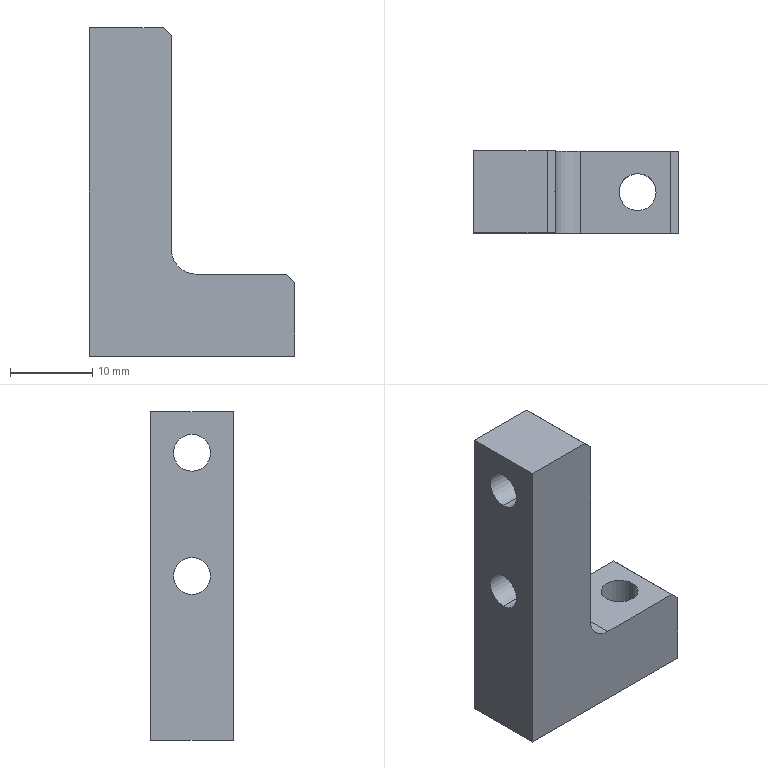Part | SolidWorks | features HoleWzd 2, Chamfer 1, Extrusion 1, ICE 1 | 1 solid | 23 faces | box 25 x 10 x 40 mm | volume 4716 mm3 | plane 12 | cylinder 11 | commonest cylinder face diameters 4.5 x6 8 x4 6 x1
STEP:
#1=CARTESIAN_POINT('',(5.25,0.,-20.));
#2=VERTEX_POINT('',#1);
#3=CARTESIAN_POINT('',(9.75,0.,-20.));
#4=VERTEX_POINT('',#3);
#5=CARTESIAN_POINT('',(7.5,0.,-20.));
#6=DIRECTION('',(0.,0.,1.));
#7=DIRECTION('',(1.,0.,0.));
#8=AXIS2_PLACEMENT_3D('',#5,#6,#7);
#9=CIRCLE('',#8,2.25);
#10=EDGE_CURVE('',#2,#4,#9,.T.);
#11=ORIENTED_EDGE('',*,*,#10,.F.);
#12=CARTESIAN_POINT('',(5.25,0.,-10.));
#13=VERTEX_POINT('',#12);
#14=CARTESIAN_POINT('',(5.25,0.,-10.));
#15=DIRECTION('',(0.,0.,1.));
#16=VECTOR('',#15,1000.);
#17=LINE('',#14,#16);
#18=EDGE_CURVE('',#2,#13,#17,.T.);
#19=ORIENTED_EDGE('',*,*,#18,.T.);
#20=CARTESIAN_POINT('',(9.75,0.,-10.));
#21=VERTEX_POINT('',#20);
#22=CARTESIAN_POINT('',(7.5,0.,-10.));
#23=DIRECTION('',(0.,0.,1.));
#24=DIRECTION('',(1.,0.,0.));
#25=AXIS2_PLACEMENT_3D('',#22,#23,#24);
#26=CIRCLE('',#25,2.25);
#27=EDGE_CURVE('',#13,#21,#26,.T.);
#28=ORIENTED_EDGE('',*,*,#27,.T.);
#29=CARTESIAN_POINT('',(9.75,0.,-10.));
#30=DIRECTION('',(0.,0.,1.));
#31=VECTOR('',#30,1000.);
#32=LINE('',#29,#31);
#33=EDGE_CURVE('',#4,#21,#32,.T.);
#34=ORIENTED_EDGE('',*,*,#33,.F.);
#35=EDGE_LOOP('',(#11,#19,#28,#34));
#36=FACE_OUTER_BOUND('',#35,.T.);
#37=CARTESIAN_POINT('',(7.5,0.,-10.));
#38=DIRECTION('',(0.,0.,1.));
#39=DIRECTION('',(1.,0.,0.));
#40=AXIS2_PLACEMENT_3D('',#37,#38,#39);
#41=CYLINDRICAL_SURFACE('',#40,2.25);
#42=ADVANCED_FACE('',(#36),#41,.F.);
#43=CARTESIAN_POINT('',(-7.1,0.,19.));
#44=VERTEX_POINT('',#43);
#45=CARTESIAN_POINT('',(-7.1,0.,11.));
#46=VERTEX_POINT('',#45);
#47=CARTESIAN_POINT('',(-7.1,0.,15.));
#48=DIRECTION('',(1.,0.,0.));
#49=DIRECTION('',(0.,0.,-1.));
#50=AXIS2_PLACEMENT_3D('',#47,#48,#49);
#51=CIRCLE('',#50,4.);
#52=EDGE_CURVE('',#44,#46,#51,.T.);
#53=ORIENTED_EDGE('',*,*,#52,.F.);
#54=CARTESIAN_POINT('',(-2.5,0.,19.));
#55=VERTEX_POINT('',#54);
#56=CARTESIAN_POINT('',(-2.5,0.,19.));
#57=DIRECTION('',(1.,0.,0.));
#58=VECTOR('',#57,1000.);
#59=LINE('',#56,#58);
#60=EDGE_CURVE('',#44,#55,#59,.T.);
#61=ORIENTED_EDGE('',*,*,#60,.T.);
#62=CARTESIAN_POINT('',(-2.5,0.,11.));
#63=VERTEX_POINT('',#62);
#64=CARTESIAN_POINT('',(-2.5,0.,15.));
#65=DIRECTION('',(1.,0.,0.));
#66=DIRECTION('',(0.,0.,-1.));
#67=AXIS2_PLACEMENT_3D('',#64,#65,#66);
#68=CIRCLE('',#67,4.);
#69=EDGE_CURVE('',#55,#63,#68,.T.);
#70=ORIENTED_EDGE('',*,*,#69,.T.);
#71=CARTESIAN_POINT('',(-2.5,0.,11.));
#72=DIRECTION('',(1.,0.,0.));
#73=VECTOR('',#72,1000.);
#74=LINE('',#71,#73);
#75=EDGE_CURVE('',#46,#63,#74,.T.);
#76=ORIENTED_EDGE('',*,*,#75,.F.);
#77=EDGE_LOOP('',(#53,#61,#70,#76));
#78=FACE_OUTER_BOUND('',#77,.T.);
#79=CARTESIAN_POINT('',(-2.5,0.,15.));
#80=DIRECTION('',(1.,0.,0.));
#81=DIRECTION('',(0.,0.,-1.));
#82=AXIS2_PLACEMENT_3D('',#79,#80,#81);
#83=CYLINDRICAL_SURFACE('',#82,4.);
#84=ADVANCED_FACE('',(#78),#83,.F.);
#85=CARTESIAN_POINT('',(-12.5,0.,17.25));
#86=VERTEX_POINT('',#85);
#87=CARTESIAN_POINT('',(-12.5,0.,12.75));
#88=VERTEX_POINT('',#87);
#89=CARTESIAN_POINT('',(-12.5,0.,15.));
#90=DIRECTION('',(1.,0.,0.));
#91=DIRECTION('',(0.,0.,-1.));
#92=AXIS2_PLACEMENT_3D('',#89,#90,#91);
#93=CIRCLE('',#92,2.25);
#94=EDGE_CURVE('',#86,#88,#93,.T.);
#95=ORIENTED_EDGE('',*,*,#94,.F.);
#96=CARTESIAN_POINT('',(-7.1,0.,17.25));
#97=VERTEX_POINT('',#96);
#98=CARTESIAN_POINT('',(-2.5,0.,17.25));
#99=DIRECTION('',(1.,0.,0.));
#100=VECTOR('',#99,1000.);
#101=LINE('',#98,#100);
#102=EDGE_CURVE('',#86,#97,#101,.T.);
#103=ORIENTED_EDGE('',*,*,#102,.T.);
#104=CARTESIAN_POINT('',(-7.1,0.,12.75));
#105=VERTEX_POINT('',#104);
#106=CARTESIAN_POINT('',(-7.1,0.,15.));
#107=DIRECTION('',(1.,0.,0.));
#108=DIRECTION('',(0.,0.,-1.));
#109=AXIS2_PLACEMENT_3D('',#106,#107,#108);
#110=CIRCLE('',#109,2.25);
#111=EDGE_CURVE('',#97,#105,#110,.T.);
#112=ORIENTED_EDGE('',*,*,#111,.T.);
#113=CARTESIAN_POINT('',(-2.5,0.,12.75));
#114=DIRECTION('',(1.,0.,0.));
#115=VECTOR('',#114,1000.);
#116=LINE('',#113,#115);
#117=EDGE_CURVE('',#88,#105,#116,.T.);
#118=ORIENTED_EDGE('',*,*,#117,.F.);
#119=EDGE_LOOP('',(#95,#103,#112,#118));
#120=FACE_OUTER_BOUND('',#119,.T.);
#121=CARTESIAN_POINT('',(-2.5,0.,15.));
#122=DIRECTION('',(1.,0.,0.));
#123=DIRECTION('',(0.,0.,-1.));
#124=AXIS2_PLACEMENT_3D('',#121,#122,#123);
#125=CYLINDRICAL_SURFACE('',#124,2.25);
#126=ADVANCED_FACE('',(#120),#125,.F.);
#127=CARTESIAN_POINT('',(-7.1,0.,4.));
#128=VERTEX_POINT('',#127);
#129=CARTESIAN_POINT('',(-7.1,0.,-4.));
#130=VERTEX_POINT('',#129);
#131=CARTESIAN_POINT('',(-7.1,0.,0.));
#132=DIRECTION('',(1.,0.,0.));
#133=DIRECTION('',(0.,0.,-1.));
#134=AXIS2_PLACEMENT_3D('',#131,#132,#133);
#135=CIRCLE('',#134,4.);
#136=EDGE_CURVE('',#128,#130,#135,.T.);
#137=ORIENTED_EDGE('',*,*,#136,.F.);
#138=CARTESIAN_POINT('',(-2.5,0.,4.));
#139=VERTEX_POINT('',#138);
#140=CARTESIAN_POINT('',(-2.5,0.,4.));
#141=DIRECTION('',(1.,0.,0.));
#142=VECTOR('',#141,1000.);
#143=LINE('',#140,#142);
#144=EDGE_CURVE('',#128,#139,#143,.T.);
#145=ORIENTED_EDGE('',*,*,#144,.T.);
#146=CARTESIAN_POINT('',(-2.5,0.,-4.));
#147=VERTEX_POINT('',#146);
#148=CARTESIAN_POINT('',(-2.5,0.,0.));
#149=DIRECTION('',(1.,0.,0.));
#150=DIRECTION('',(0.,0.,-1.));
#151=AXIS2_PLACEMENT_3D('',#148,#149,#150);
#152=CIRCLE('',#151,4.);
#153=EDGE_CURVE('',#139,#147,#152,.T.);
#154=ORIENTED_EDGE('',*,*,#153,.T.);
#155=CARTESIAN_POINT('',(-2.5,0.,-4.));
#156=DIRECTION('',(1.,0.,0.));
#157=VECTOR('',#156,1000.);
#158=LINE('',#155,#157);
#159=EDGE_CURVE('',#130,#147,#158,.T.);
#160=ORIENTED_EDGE('',*,*,#159,.F.);
#161=EDGE_LOOP('',(#137,#145,#154,#160));
#162=FACE_OUTER_BOUND('',#161,.T.);
#163=CARTESIAN_POINT('',(-2.5,0.,0.));
#164=DIRECTION('',(1.,0.,0.));
#165=DIRECTION('',(0.,0.,-1.));
#166=AXIS2_PLACEMENT_3D('',#163,#164,#165);
#167=CYLINDRICAL_SURFACE('',#166,4.);
#168=ADVANCED_FACE('',(#162),#167,.F.);
#169=CARTESIAN_POINT('',(-12.5,0.,2.25));
#170=VERTEX_POINT('',#169);
#171=CARTESIAN_POINT('',(-12.5,0.,-2.25));
#172=VERTEX_POINT('',#171);
#173=CARTESIAN_POINT('',(-12.5,0.,0.));
#174=DIRECTION('',(1.,0.,0.));
#175=DIRECTION('',(0.,0.,-1.));
#176=AXIS2_PLACEMENT_3D('',#173,#174,#175);
#177=CIRCLE('',#176,2.25);
#178=EDGE_CURVE('',#170,#172,#177,.T.);
#179=ORIENTED_EDGE('',*,*,#178,.F.);
#180=CARTESIAN_POINT('',(-7.1,0.,2.25));
#181=VERTEX_POINT('',#180);
#182=CARTESIAN_POINT('',(-2.5,0.,2.25));
#183=DIRECTION('',(1.,0.,0.));
#184=VECTOR('',#183,1000.);
#185=LINE('',#182,#184);
#186=EDGE_CURVE('',#170,#181,#185,.T.);
#187=ORIENTED_EDGE('',*,*,#186,.T.);
#188=CARTESIAN_POINT('',(-7.1,0.,-2.25));
#189=VERTEX_POINT('',#188);
#190=CARTESIAN_POINT('',(-7.1,0.,0.));
#191=DIRECTION('',(1.,0.,0.));
#192=DIRECTION('',(0.,0.,-1.));
#193=AXIS2_PLACEMENT_3D('',#190,#191,#192);
#194=CIRCLE('',#193,2.25);
#195=EDGE_CURVE('',#181,#189,#194,.T.);
#196=ORIENTED_EDGE('',*,*,#195,.T.);
#197=CARTESIAN_POINT('',(-2.5,0.,-2.25));
#198=DIRECTION('',(1.,0.,0.));
#199=VECTOR('',#198,1000.);
#200=LINE('',#197,#199);
#201=EDGE_CURVE('',#172,#189,#200,.T.);
#202=ORIENTED_EDGE('',*,*,#201,.F.);
#203=EDGE_LOOP('',(#179,#187,#196,#202));
#204=FACE_OUTER_BOUND('',#203,.T.);
#205=CARTESIAN_POINT('',(-2.5,0.,0.));
#206=DIRECTION('',(1.,0.,0.));
#207=DIRECTION('',(0.,0.,-1.));
#208=AXIS2_PLACEMENT_3D('',#205,#206,#207);
#209=CYLINDRICAL_SURFACE('',#208,2.25);
#210=ADVANCED_FACE('',(#204),#209,.F.);
#211=CARTESIAN_POINT('',(12.5,5.,-11.));
#212=VERTEX_POINT('',#211);
#213=CARTESIAN_POINT('',(12.5,5.,-20.));
#214=VERTEX_POINT('',#213);
#215=CARTESIAN_POINT('',(12.5,5.,20.));
#216=DIRECTION('',(0.,0.,-1.));
#217=VECTOR('',#216,1000.);
#218=LINE('',#215,#217);
#219=EDGE_CURVE('',#212,#214,#218,.T.);
#220=ORIENTED_EDGE('',*,*,#219,.F.);
#221=CARTESIAN_POINT('',(12.5,-5.,-11.));
#222=VERTEX_POINT('',#221);
#223=CARTESIAN_POINT('',(12.5,5.,-11.));
#224=DIRECTION('',(0.,-1.,0.));
#225=VECTOR('',#224,1000.);
#226=LINE('',#223,#225);
#227=EDGE_CURVE('',#212,#222,#226,.T.);
#228=ORIENTED_EDGE('',*,*,#227,.T.);
#229=CARTESIAN_POINT('',(12.5,-5.,-20.));
#230=VERTEX_POINT('',#229);
#231=CARTESIAN_POINT('',(12.5,-5.,20.));
#232=DIRECTION('',(0.,0.,-1.));
#233=VECTOR('',#232,1000.);
#234=LINE('',#231,#233);
#235=EDGE_CURVE('',#222,#230,#234,.T.);
#236=ORIENTED_EDGE('',*,*,#235,.T.);
#237=CARTESIAN_POINT('',(12.5,5.,-20.));
#238=DIRECTION('',(0.,-1.,0.));
#239=VECTOR('',#238,1000.);
#240=LINE('',#237,#239);
#241=EDGE_CURVE('',#214,#230,#240,.T.);
#242=ORIENTED_EDGE('',*,*,#241,.F.);
#243=EDGE_LOOP('',(#220,#228,#236,#242));
#244=FACE_OUTER_BOUND('',#243,.T.);
#245=CARTESIAN_POINT('',(12.5,5.,20.));
#246=DIRECTION('',(-1.,0.,0.));
#247=DIRECTION('',(0.,0.,1.));
#248=AXIS2_PLACEMENT_3D('',#245,#246,#247);
#249=PLANE('',#248);
#250=ADVANCED_FACE('',(#244),#249,.F.);
#251=CARTESIAN_POINT('',(7.5,0.,-20.));
#252=DIRECTION('',(0.,0.,1.));
#253=DIRECTION('',(1.,0.,0.));
#254=AXIS2_PLACEMENT_3D('',#251,#252,#253);
#255=CIRCLE('',#254,2.25);
#256=EDGE_CURVE('',#4,#2,#255,.T.);
#257=ORIENTED_EDGE('',*,*,#256,.T.);
#258=ORIENTED_EDGE('',*,*,#10,.T.);
#259=EDGE_LOOP('',(#257,#258));
#260=FACE_BOUND('',#259,.T.);
#261=CARTESIAN_POINT('',(-12.5,-5.,-20.));
#262=VERTEX_POINT('',#261);
#263=CARTESIAN_POINT('',(-12.5,-5.,-20.));
#264=DIRECTION('',(-1.,0.,0.));
#265=VECTOR('',#264,1000.);
#266=LINE('',#263,#265);
#267=EDGE_CURVE('',#230,#262,#266,.T.);
#268=ORIENTED_EDGE('',*,*,#267,.T.);
#269=CARTESIAN_POINT('',(-12.5,5.,-20.));
#270=VERTEX_POINT('',#269);
#271=CARTESIAN_POINT('',(-12.5,5.,-20.));
#272=DIRECTION('',(0.,-1.,0.));
#273=VECTOR('',#272,1000.);
#274=LINE('',#271,#273);
#275=EDGE_CURVE('',#270,#262,#274,.T.);
#276=ORIENTED_EDGE('',*,*,#275,.F.);
#277=CARTESIAN_POINT('',(-12.5,5.,-20.));
#278=DIRECTION('',(-1.,0.,0.));
#279=VECTOR('',#278,1000.);
#280=LINE('',#277,#279);
#281=EDGE_CURVE('',#214,#270,#280,.T.);
#282=ORIENTED_EDGE('',*,*,#281,.F.);
#283=ORIENTED_EDGE('',*,*,#241,.T.);
#284=EDGE_LOOP('',(#268,#276,#282,#283));
#285=FACE_OUTER_BOUND('',#284,.T.);
#286=CARTESIAN_POINT('',(-12.5,5.,-20.));
#287=DIRECTION('',(0.,0.,1.));
#288=DIRECTION('',(1.,0.,0.));
#289=AXIS2_PLACEMENT_3D('',#286,#287,#288);
#290=PLANE('',#289);
#291=ADVANCED_FACE('',(#260,#285),#290,.F.);
#292=CARTESIAN_POINT('',(-12.5,0.,15.));
#293=DIRECTION('',(1.,0.,0.));
#294=DIRECTION('',(0.,0.,-1.));
#295=AXIS2_PLACEMENT_3D('',#292,#293,#294);
#296=CIRCLE('',#295,2.25);
#297=EDGE_CURVE('',#88,#86,#296,.T.);
#298=ORIENTED_EDGE('',*,*,#297,.T.);
#299=ORIENTED_EDGE('',*,*,#94,.T.);
#300=EDGE_LOOP('',(#298,#299));
#301=FACE_BOUND('',#300,.T.);
#302=CARTESIAN_POINT('',(-12.5,0.,0.));
#303=DIRECTION('',(1.,0.,0.));
#304=DIRECTION('',(0.,0.,-1.));
#305=AXIS2_PLACEMENT_3D('',#302,#303,#304);
#306=CIRCLE('',#305,2.25);
#307=EDGE_CURVE('',#172,#170,#306,.T.);
#308=ORIENTED_EDGE('',*,*,#307,.T.);
#309=ORIENTED_EDGE('',*,*,#178,.T.);
#310=EDGE_LOOP('',(#308,#309));
#311=FACE_BOUND('',#310,.T.);
#312=CARTESIAN_POINT('',(-12.5,-5.,20.));
#313=VERTEX_POINT('',#312);
#314=CARTESIAN_POINT('',(-12.5,-5.,20.));
#315=DIRECTION('',(0.,0.,1.));
#316=VECTOR('',#315,1000.);
#317=LINE('',#314,#316);
#318=EDGE_CURVE('',#262,#313,#317,.T.);
#319=ORIENTED_EDGE('',*,*,#318,.T.);
#320=CARTESIAN_POINT('',(-12.5,5.,20.));
#321=VERTEX_POINT('',#320);
#322=CARTESIAN_POINT('',(-12.5,5.,20.));
#323=DIRECTION('',(0.,-1.,0.));
#324=VECTOR('',#323,1000.);
#325=LINE('',#322,#324);
#326=EDGE_CURVE('',#321,#313,#325,.T.);
#327=ORIENTED_EDGE('',*,*,#326,.F.);
#328=CARTESIAN_POINT('',(-12.5,5.,20.));
#329=DIRECTION('',(0.,0.,1.));
#330=VECTOR('',#329,1000.);
#331=LINE('',#328,#330);
#332=EDGE_CURVE('',#270,#321,#331,.T.);
#333=ORIENTED_EDGE('',*,*,#332,.F.);
#334=ORIENTED_EDGE('',*,*,#275,.T.);
#335=EDGE_LOOP('',(#319,#327,#333,#334));
#336=FACE_OUTER_BOUND('',#335,.T.);
#337=CARTESIAN_POINT('',(-12.5,5.,20.));
#338=DIRECTION('',(1.,0.,0.));
#339=DIRECTION('',(0.,0.,-1.));
#340=AXIS2_PLACEMENT_3D('',#337,#338,#339);
#341=PLANE('',#340);
#342=ADVANCED_FACE('',(#301,#311,#336),#341,.F.);
#343=CARTESIAN_POINT('',(-3.5,-5.,20.));
#344=VERTEX_POINT('',#343);
#345=CARTESIAN_POINT('',(-12.5,-5.,20.));
#346=DIRECTION('',(1.,0.,0.));
#347=VECTOR('',#346,1000.);
#348=LINE('',#345,#347);
#349=EDGE_CURVE('',#313,#344,#348,.T.);
#350=ORIENTED_EDGE('',*,*,#349,.T.);
#351=CARTESIAN_POINT('',(-3.5,5.,20.));
#352=VERTEX_POINT('',#351);
#353=CARTESIAN_POINT('',(-3.5,5.,20.));
#354=DIRECTION('',(0.,1.,0.));
#355=VECTOR('',#354,1000.);
#356=LINE('',#353,#355);
#357=EDGE_CURVE('',#344,#352,#356,.T.);
#358=ORIENTED_EDGE('',*,*,#357,.T.);
#359=CARTESIAN_POINT('',(-12.5,5.,20.));
#360=DIRECTION('',(1.,0.,0.));
#361=VECTOR('',#360,1000.);
#362=LINE('',#359,#361);
#363=EDGE_CURVE('',#321,#352,#362,.T.);
#364=ORIENTED_EDGE('',*,*,#363,.F.);
#365=ORIENTED_EDGE('',*,*,#326,.T.);
#366=EDGE_LOOP('',(#350,#358,#364,#365));
#367=FACE_OUTER_BOUND('',#366,.T.);
#368=CARTESIAN_POINT('',(-12.5,5.,20.));
#369=DIRECTION('',(0.,0.,-1.));
#370=DIRECTION('',(-1.,0.,0.));
#371=AXIS2_PLACEMENT_3D('',#368,#369,#370);
#372=PLANE('',#371);
#373=ADVANCED_FACE('',(#367),#372,.F.);
#374=ORIENTED_EDGE('',*,*,#363,.T.);
#375=CARTESIAN_POINT('',(-2.5,5.,19.));
#376=VERTEX_POINT('',#375);
#377=CARTESIAN_POINT('',(-3.5,5.,20.));
#378=DIRECTION('',(0.7071,0.,-0.7071));
#379=VECTOR('',#378,1000.);
#380=LINE('',#377,#379);
#381=EDGE_CURVE('',#352,#376,#380,.T.);
#382=ORIENTED_EDGE('',*,*,#381,.T.);
#383=CARTESIAN_POINT('',(-2.5,5.,-7.));
#384=VERTEX_POINT('',#383);
#385=CARTESIAN_POINT('',(-2.5,5.,20.));
#386=DIRECTION('',(0.,0.,1.));
#387=VECTOR('',#386,1000.);
#388=LINE('',#385,#387);
#389=EDGE_CURVE('',#384,#376,#388,.T.);
#390=ORIENTED_EDGE('',*,*,#389,.F.);
#391=CARTESIAN_POINT('',(0.5,5.,-10.));
#392=VERTEX_POINT('',#391);
#393=CARTESIAN_POINT('',(0.5,5.,-7.));
#394=DIRECTION('',(0.,1.,0.));
#395=DIRECTION('',(0.,0.,1.));
#396=AXIS2_PLACEMENT_3D('',#393,#394,#395);
#397=CIRCLE('',#396,3.);
#398=EDGE_CURVE('',#392,#384,#397,.T.);
#399=ORIENTED_EDGE('',*,*,#398,.F.);
#400=CARTESIAN_POINT('',(11.5,5.,-10.));
#401=VERTEX_POINT('',#400);
#402=CARTESIAN_POINT('',(12.5,5.,-10.));
#403=DIRECTION('',(-1.,0.,0.));
#404=VECTOR('',#403,1000.);
#405=LINE('',#402,#404);
#406=EDGE_CURVE('',#401,#392,#405,.T.);
#407=ORIENTED_EDGE('',*,*,#406,.F.);
#408=CARTESIAN_POINT('',(11.5,5.,-10.));
#409=DIRECTION('',(0.7071,0.,-0.7071));
#410=VECTOR('',#409,1000.);
#411=LINE('',#408,#410);
#412=EDGE_CURVE('',#401,#212,#411,.T.);
#413=ORIENTED_EDGE('',*,*,#412,.T.);
#414=ORIENTED_EDGE('',*,*,#219,.T.);
#415=ORIENTED_EDGE('',*,*,#281,.T.);
#416=ORIENTED_EDGE('',*,*,#332,.T.);
#417=EDGE_LOOP('',(#374,#382,#390,#399,#407,#413,#414,#415,#416));
#418=FACE_OUTER_BOUND('',#417,.T.);
#419=CARTESIAN_POINT('',(0.,5.,0.));
#420=DIRECTION('',(0.,-1.,0.));
#421=DIRECTION('',(0.,0.,-1.));
#422=AXIS2_PLACEMENT_3D('',#419,#420,#421);
#423=PLANE('',#422);
#424=ADVANCED_FACE('',(#418),#423,.F.);
#425=CARTESIAN_POINT('',(-2.5,-5.,-7.));
#426=VERTEX_POINT('',#425);
#427=CARTESIAN_POINT('',(-2.5,-5.,19.));
#428=VERTEX_POINT('',#427);
#429=CARTESIAN_POINT('',(-2.5,-5.,20.));
#430=DIRECTION('',(0.,0.,1.));
#431=VECTOR('',#430,1000.);
#432=LINE('',#429,#431);
#433=EDGE_CURVE('',#426,#428,#432,.T.);
#434=ORIENTED_EDGE('',*,*,#433,.T.);
#435=CARTESIAN_POINT('',(8.25,-5.,8.25));
#436=DIRECTION('',(-0.7071,0.,0.7071));
#437=VECTOR('',#436,1000.);
#438=LINE('',#435,#437);
#439=EDGE_CURVE('',#428,#344,#438,.T.);
#440=ORIENTED_EDGE('',*,*,#439,.T.);
#441=ORIENTED_EDGE('',*,*,#349,.F.);
#442=ORIENTED_EDGE('',*,*,#318,.F.);
#443=ORIENTED_EDGE('',*,*,#267,.F.);
#444=ORIENTED_EDGE('',*,*,#235,.F.);
#445=CARTESIAN_POINT('',(11.5,-5.,-10.));
#446=VERTEX_POINT('',#445);
#447=CARTESIAN_POINT('',(0.75,-5.,0.75));
#448=DIRECTION('',(-0.7071,0.,0.7071));
#449=VECTOR('',#448,1000.);
#450=LINE('',#447,#449);
#451=EDGE_CURVE('',#222,#446,#450,.T.);
#452=ORIENTED_EDGE('',*,*,#451,.T.);
#453=CARTESIAN_POINT('',(0.5,-5.,-10.));
#454=VERTEX_POINT('',#453);
#455=CARTESIAN_POINT('',(12.5,-5.,-10.));
#456=DIRECTION('',(-1.,0.,0.));
#457=VECTOR('',#456,1000.);
#458=LINE('',#455,#457);
#459=EDGE_CURVE('',#446,#454,#458,.T.);
#460=ORIENTED_EDGE('',*,*,#459,.T.);
#461=CARTESIAN_POINT('',(0.5,-5.,-7.));
#462=DIRECTION('',(0.,1.,0.));
#463=DIRECTION('',(0.,0.,-1.));
#464=AXIS2_PLACEMENT_3D('',#461,#462,#463);
#465=CIRCLE('',#464,3.);
#466=EDGE_CURVE('',#454,#426,#465,.T.);
#467=ORIENTED_EDGE('',*,*,#466,.T.);
#468=EDGE_LOOP('',(#434,#440,#441,#442,#443,#444,#452,#460,#467));
#469=FACE_OUTER_BOUND('',#468,.T.);
#470=CARTESIAN_POINT('',(0.,-5.,0.));
#471=DIRECTION('',(0.,-1.,0.));
#472=DIRECTION('',(0.,0.,-1.));
#473=AXIS2_PLACEMENT_3D('',#470,#471,#472);
#474=PLANE('',#473);
#475=ADVANCED_FACE('',(#469),#474,.T.);
#476=CARTESIAN_POINT('',(7.5,0.,-10.));
#477=DIRECTION('',(0.,0.,1.));
#478=DIRECTION('',(1.,0.,0.));
#479=AXIS2_PLACEMENT_3D('',#476,#477,#478);
#480=CIRCLE('',#479,2.25);
#481=EDGE_CURVE('',#21,#13,#480,.T.);
#482=ORIENTED_EDGE('',*,*,#481,.F.);
#483=ORIENTED_EDGE('',*,*,#27,.F.);
#484=EDGE_LOOP('',(#482,#483));
#485=FACE_BOUND('',#484,.T.);
#486=ORIENTED_EDGE('',*,*,#459,.F.);
#487=CARTESIAN_POINT('',(11.5,-38.541,-10.));
#488=DIRECTION('',(0.,1.,0.));
#489=VECTOR('',#488,1000.);
#490=LINE('',#487,#489);
#491=EDGE_CURVE('',#446,#401,#490,.T.);
#492=ORIENTED_EDGE('',*,*,#491,.T.);
#493=ORIENTED_EDGE('',*,*,#406,.T.);
#494=CARTESIAN_POINT('',(0.5,-38.541,-10.));
#495=DIRECTION('',(0.,1.,0.));
#496=VECTOR('',#495,1000.);
#497=LINE('',#494,#496);
#498=EDGE_CURVE('',#454,#392,#497,.T.);
#499=ORIENTED_EDGE('',*,*,#498,.F.);
#500=EDGE_LOOP('',(#486,#492,#493,#499));
#501=FACE_OUTER_BOUND('',#500,.T.);
#502=CARTESIAN_POINT('',(12.5,-38.541,-10.));
#503=DIRECTION('',(0.,0.,-1.));
#504=DIRECTION('',(-1.,0.,0.));
#505=AXIS2_PLACEMENT_3D('',#502,#503,#504);
#506=PLANE('',#505);
#507=ADVANCED_FACE('',(#485,#501),#506,.F.);
#508=ORIENTED_EDGE('',*,*,#498,.T.);
#509=ORIENTED_EDGE('',*,*,#398,.T.);
#510=CARTESIAN_POINT('',(-2.5,-38.541,-7.));
#511=DIRECTION('',(0.,1.,0.));
#512=VECTOR('',#511,1000.);
#513=LINE('',#510,#512);
#514=EDGE_CURVE('',#426,#384,#513,.T.);
#515=ORIENTED_EDGE('',*,*,#514,.F.);
#516=ORIENTED_EDGE('',*,*,#466,.F.);
#517=EDGE_LOOP('',(#508,#509,#515,#516));
#518=FACE_OUTER_BOUND('',#517,.T.);
#519=CARTESIAN_POINT('',(0.5,-38.541,-7.));
#520=DIRECTION('',(0.,1.,0.));
#521=DIRECTION('',(0.,0.,1.));
#522=AXIS2_PLACEMENT_3D('',#519,#520,#521);
#523=CYLINDRICAL_SURFACE('',#522,3.);
#524=ADVANCED_FACE('',(#518),#523,.F.);
#525=CARTESIAN_POINT('',(-2.5,0.,0.));
#526=DIRECTION('',(1.,0.,0.));
#527=DIRECTION('',(0.,0.,-1.));
#528=AXIS2_PLACEMENT_3D('',#525,#526,#527);
#529=CIRCLE('',#528,4.);
#530=EDGE_CURVE('',#147,#139,#529,.T.);
#531=ORIENTED_EDGE('',*,*,#530,.F.);
#532=ORIENTED_EDGE('',*,*,#153,.F.);
#533=EDGE_LOOP('',(#531,#532));
#534=FACE_BOUND('',#533,.T.);
#535=CARTESIAN_POINT('',(-2.5,-38.541,19.));
#536=DIRECTION('',(0.,-1.,0.));
#537=VECTOR('',#536,1000.);
#538=LINE('',#535,#537);
#539=EDGE_CURVE('',#376,#55,#538,.T.);
#540=ORIENTED_EDGE('',*,*,#539,.T.);
#541=CARTESIAN_POINT('',(-2.5,0.,15.));
#542=DIRECTION('',(1.,0.,0.));
#543=DIRECTION('',(0.,0.,-1.));
#544=AXIS2_PLACEMENT_3D('',#541,#542,#543);
#545=CIRCLE('',#544,4.);
#546=EDGE_CURVE('',#63,#55,#545,.T.);
#547=ORIENTED_EDGE('',*,*,#546,.F.);
#548=ORIENTED_EDGE('',*,*,#69,.F.);
#549=CARTESIAN_POINT('',(-2.5,-38.541,19.));
#550=DIRECTION('',(0.,-1.,0.));
#551=VECTOR('',#550,1000.);
#552=LINE('',#549,#551);
#553=EDGE_CURVE('',#55,#428,#552,.T.);
#554=ORIENTED_EDGE('',*,*,#553,.T.);
#555=ORIENTED_EDGE('',*,*,#433,.F.);
#556=ORIENTED_EDGE('',*,*,#514,.T.);
#557=ORIENTED_EDGE('',*,*,#389,.T.);
#558=EDGE_LOOP('',(#540,#547,#548,#554,#555,#556,#557));
#559=FACE_OUTER_BOUND('',#558,.T.);
#560=CARTESIAN_POINT('',(-2.5,-38.541,20.));
#561=DIRECTION('',(-1.,0.,0.));
#562=DIRECTION('',(0.,0.,1.));
#563=AXIS2_PLACEMENT_3D('',#560,#561,#562);
#564=PLANE('',#563);
#565=ADVANCED_FACE('',(#534,#559),#564,.F.);
#566=ORIENTED_EDGE('',*,*,#439,.F.);
#567=ORIENTED_EDGE('',*,*,#553,.F.);
#568=ORIENTED_EDGE('',*,*,#539,.F.);
#569=ORIENTED_EDGE('',*,*,#381,.F.);
#570=ORIENTED_EDGE('',*,*,#357,.F.);
#571=EDGE_LOOP('',(#566,#567,#568,#569,#570));
#572=FACE_OUTER_BOUND('',#571,.T.);
#573=CARTESIAN_POINT('',(-3.5,5.,20.));
#574=DIRECTION('',(-0.7071,0.,-0.7071));
#575=DIRECTION('',(0.,1.,0.));
#576=AXIS2_PLACEMENT_3D('',#573,#574,#575);
#577=PLANE('',#576);
#578=ADVANCED_FACE('',(#572),#577,.F.);
#579=ORIENTED_EDGE('',*,*,#451,.F.);
#580=ORIENTED_EDGE('',*,*,#227,.F.);
#581=ORIENTED_EDGE('',*,*,#412,.F.);
#582=ORIENTED_EDGE('',*,*,#491,.F.);
#583=EDGE_LOOP('',(#579,#580,#581,#582));
#584=FACE_OUTER_BOUND('',#583,.T.);
#585=CARTESIAN_POINT('',(11.5,-38.541,-10.));
#586=DIRECTION('',(-0.7071,0.,-0.7071));
#587=DIRECTION('',(0.,1.,0.));
#588=AXIS2_PLACEMENT_3D('',#585,#586,#587);
#589=PLANE('',#588);
#590=ADVANCED_FACE('',(#584),#589,.F.);
#591=ORIENTED_EDGE('',*,*,#186,.F.);
#592=ORIENTED_EDGE('',*,*,#307,.F.);
#593=ORIENTED_EDGE('',*,*,#201,.T.);
#594=CARTESIAN_POINT('',(-7.1,0.,0.));
#595=DIRECTION('',(1.,0.,0.));
#596=DIRECTION('',(0.,0.,-1.));
#597=AXIS2_PLACEMENT_3D('',#594,#595,#596);
#598=CIRCLE('',#597,2.25);
#599=EDGE_CURVE('',#189,#181,#598,.T.);
#600=ORIENTED_EDGE('',*,*,#599,.T.);
#601=EDGE_LOOP('',(#591,#592,#593,#600));
#602=FACE_OUTER_BOUND('',#601,.T.);
#603=CARTESIAN_POINT('',(-2.5,0.,0.));
#604=DIRECTION('',(1.,0.,0.));
#605=DIRECTION('',(0.,0.,-1.));
#606=AXIS2_PLACEMENT_3D('',#603,#604,#605);
#607=CYLINDRICAL_SURFACE('',#606,2.25);
#608=ADVANCED_FACE('',(#602),#607,.F.);
#609=ORIENTED_EDGE('',*,*,#599,.F.);
#610=ORIENTED_EDGE('',*,*,#195,.F.);
#611=EDGE_LOOP('',(#609,#610));
#612=FACE_BOUND('',#611,.T.);
#613=CARTESIAN_POINT('',(-7.1,0.,0.));
#614=DIRECTION('',(1.,0.,0.));
#615=DIRECTION('',(0.,0.,-1.));
#616=AXIS2_PLACEMENT_3D('',#613,#614,#615);
#617=CIRCLE('',#616,4.);
#618=EDGE_CURVE('',#130,#128,#617,.T.);
#619=ORIENTED_EDGE('',*,*,#618,.T.);
#620=ORIENTED_EDGE('',*,*,#136,.T.);
#621=EDGE_LOOP('',(#619,#620));
#622=FACE_OUTER_BOUND('',#621,.T.);
#623=CARTESIAN_POINT('',(-7.1,2.25,0.));
#624=DIRECTION('',(-1.,0.,0.));
#625=DIRECTION('',(0.,0.,1.));
#626=AXIS2_PLACEMENT_3D('',#623,#624,#625);
#627=PLANE('',#626);
#628=ADVANCED_FACE('',(#612,#622),#627,.F.);
#629=ORIENTED_EDGE('',*,*,#144,.F.);
#630=ORIENTED_EDGE('',*,*,#618,.F.);
#631=ORIENTED_EDGE('',*,*,#159,.T.);
#632=ORIENTED_EDGE('',*,*,#530,.T.);
#633=EDGE_LOOP('',(#629,#630,#631,#632));
#634=FACE_OUTER_BOUND('',#633,.T.);
#635=CARTESIAN_POINT('',(-2.5,0.,0.));
#636=DIRECTION('',(1.,0.,0.));
#637=DIRECTION('',(0.,0.,-1.));
#638=AXIS2_PLACEMENT_3D('',#635,#636,#637);
#639=CYLINDRICAL_SURFACE('',#638,4.);
#640=ADVANCED_FACE('',(#634),#639,.F.);
#641=ORIENTED_EDGE('',*,*,#102,.F.);
#642=ORIENTED_EDGE('',*,*,#297,.F.);
#643=ORIENTED_EDGE('',*,*,#117,.T.);
#644=CARTESIAN_POINT('',(-7.1,0.,15.));
#645=DIRECTION('',(1.,0.,0.));
#646=DIRECTION('',(0.,0.,-1.));
#647=AXIS2_PLACEMENT_3D('',#644,#645,#646);
#648=CIRCLE('',#647,2.25);
#649=EDGE_CURVE('',#105,#97,#648,.T.);
#650=ORIENTED_EDGE('',*,*,#649,.T.);
#651=EDGE_LOOP('',(#641,#642,#643,#650));
#652=FACE_OUTER_BOUND('',#651,.T.);
#653=CARTESIAN_POINT('',(-2.5,0.,15.));
#654=DIRECTION('',(1.,0.,0.));
#655=DIRECTION('',(0.,0.,-1.));
#656=AXIS2_PLACEMENT_3D('',#653,#654,#655);
#657=CYLINDRICAL_SURFACE('',#656,2.25);
#658=ADVANCED_FACE('',(#652),#657,.F.);
#659=ORIENTED_EDGE('',*,*,#649,.F.);
#660=ORIENTED_EDGE('',*,*,#111,.F.);
#661=EDGE_LOOP('',(#659,#660));
#662=FACE_BOUND('',#661,.T.);
#663=CARTESIAN_POINT('',(-7.1,0.,15.));
#664=DIRECTION('',(1.,0.,0.));
#665=DIRECTION('',(0.,0.,-1.));
#666=AXIS2_PLACEMENT_3D('',#663,#664,#665);
#667=CIRCLE('',#666,4.);
#668=EDGE_CURVE('',#46,#44,#667,.T.);
#669=ORIENTED_EDGE('',*,*,#668,.T.);
#670=ORIENTED_EDGE('',*,*,#52,.T.);
#671=EDGE_LOOP('',(#669,#670));
#672=FACE_OUTER_BOUND('',#671,.T.);
#673=CARTESIAN_POINT('',(-7.1,2.25,15.));
#674=DIRECTION('',(-1.,0.,0.));
#675=DIRECTION('',(0.,0.,1.));
#676=AXIS2_PLACEMENT_3D('',#673,#674,#675);
#677=PLANE('',#676);
#678=ADVANCED_FACE('',(#662,#672),#677,.F.);
#679=ORIENTED_EDGE('',*,*,#60,.F.);
#680=ORIENTED_EDGE('',*,*,#668,.F.);
#681=ORIENTED_EDGE('',*,*,#75,.T.);
#682=ORIENTED_EDGE('',*,*,#546,.T.);
#683=EDGE_LOOP('',(#679,#680,#681,#682));
#684=FACE_OUTER_BOUND('',#683,.T.);
#685=CARTESIAN_POINT('',(-2.5,0.,15.));
#686=DIRECTION('',(1.,0.,0.));
#687=DIRECTION('',(0.,0.,-1.));
#688=AXIS2_PLACEMENT_3D('',#685,#686,#687);
#689=CYLINDRICAL_SURFACE('',#688,4.);
#690=ADVANCED_FACE('',(#684),#689,.F.);
#691=ORIENTED_EDGE('',*,*,#18,.F.);
#692=ORIENTED_EDGE('',*,*,#256,.F.);
#693=ORIENTED_EDGE('',*,*,#33,.T.);
#694=ORIENTED_EDGE('',*,*,#481,.T.);
#695=EDGE_LOOP('',(#691,#692,#693,#694));
#696=FACE_OUTER_BOUND('',#695,.T.);
#697=CARTESIAN_POINT('',(7.5,0.,-10.));
#698=DIRECTION('',(0.,0.,1.));
#699=DIRECTION('',(1.,0.,0.));
#700=AXIS2_PLACEMENT_3D('',#697,#698,#699);
#701=CYLINDRICAL_SURFACE('',#700,2.25);
#702=ADVANCED_FACE('',(#696),#701,.F.);
#703=CLOSED_SHELL('',(#42,#84,#126,#168,#210,#250,#291,#342,#373,#424,#475,#507,#524,#565,#578,#590,#608,#628,#640,#658,#678,#690,#702));
#704=MANIFOLD_SOLID_BREP('',#703);
#705=CARTESIAN_POINT('',(0.,0.,0.));
#706=DIRECTION('',(0.,0.,1.));
#707=DIRECTION('',(1.,0.,0.));
#708=AXIS2_PLACEMENT_3D('',#705,#706,#707);
#709=(LENGTH_UNIT()NAMED_UNIT(*)SI_UNIT(.MILLI.,.METRE.));
#710=UNCERTAINTY_MEASURE_WITH_UNIT(LENGTH_MEASURE(0.00001),#709,'','');
#711=(NAMED_UNIT(*)PLANE_ANGLE_UNIT()SI_UNIT($,.RADIAN.));
#712=(NAMED_UNIT(*)SI_UNIT($,.STERADIAN.)SOLID_ANGLE_UNIT());
#713=(GEOMETRIC_REPRESENTATION_CONTEXT(3)GLOBAL_UNCERTAINTY_ASSIGNED_CONTEXT((#710))GLOBAL_UNIT_ASSIGNED_CONTEXT((#709,#711,#712))REPRESENTATION_CONTEXT('',''));
#714=ADVANCED_BREP_SHAPE_REPRESENTATION('',(#704,#708),#713);